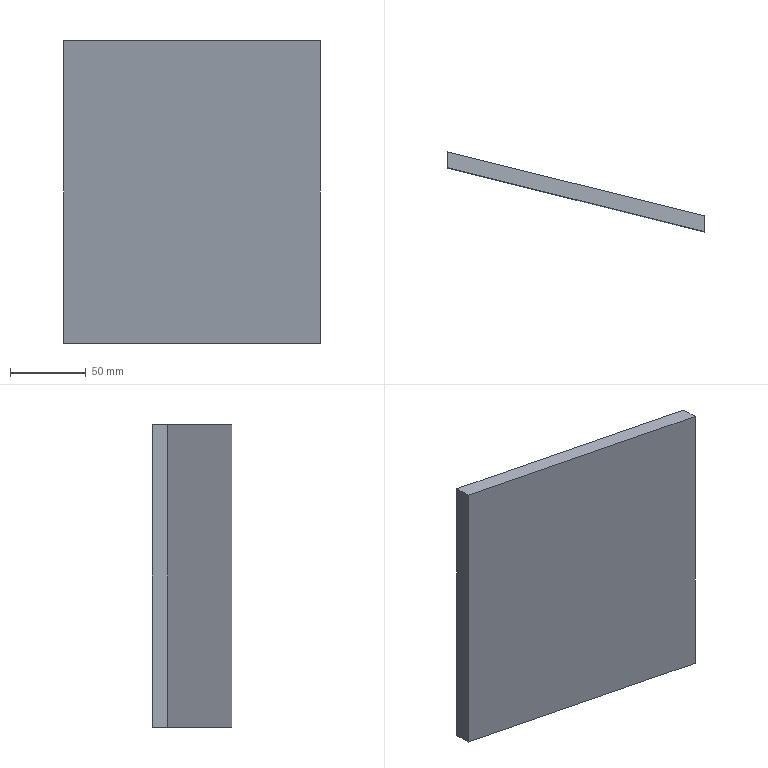Part | STEP file | 001-004-Feeding mechanism shaft slideway cover plate | 1 solid | 6 faces | box 170 x 52.886 x 200 mm | volume 357000 mm3 | plane 6
STEP:
#1=CARTESIAN_POINT('',(0.,0.,0.));
#2=DIRECTION('',(0.,0.,1.));
#3=DIRECTION('',(1.,0.,0.));
#4=AXIS2_PLACEMENT_3D('',#1,#2,#3);
#5=CARTESIAN_POINT('',(-170.,42.386,0.));
#6=VERTEX_POINT('',#5);
#7=CARTESIAN_POINT('',(0.,0.,0.));
#8=VERTEX_POINT('',#7);
#9=CARTESIAN_POINT('',(0.,0.,0.));
#10=DIRECTION('',(0.9703,-0.2419,0.));
#11=VECTOR('',#10,1.);
#12=LINE('',#9,#11);
#13=CARTESIAN_POINT('',(0.,0.,200.));
#14=DIRECTION('',(0.2419,0.9703,0.));
#15=DIRECTION('',(-0.9703,0.2419,0.));
#16=AXIS2_PLACEMENT_3D('',#13,#14,#15);
#17=PLANE('',#16);
#18=CARTESIAN_POINT('',(0.,-200.));
#19=DIRECTION('',(-1.,0.));
#20=VECTOR('',#19,1.);
#21=LINE('',#18,#20);
#22=(GEOMETRIC_REPRESENTATION_CONTEXT(2)PARAMETRIC_REPRESENTATION_CONTEXT()REPRESENTATION_CONTEXT('',''));
#23=DEFINITIONAL_REPRESENTATION('',(#21),#22);
#24=PCURVE('',#17,#23);
#25=CARTESIAN_POINT('',(0.,0.,0.));
#26=DIRECTION('',(0.,0.,-1.));
#27=DIRECTION('',(-1.,0.,0.));
#28=AXIS2_PLACEMENT_3D('',#25,#26,#27);
#29=PLANE('',#28);
#30=CARTESIAN_POINT('',(0.,0.));
#31=DIRECTION('',(-0.9703,-0.2419));
#32=VECTOR('',#31,1.);
#33=LINE('',#30,#32);
#34=(GEOMETRIC_REPRESENTATION_CONTEXT(2)PARAMETRIC_REPRESENTATION_CONTEXT()REPRESENTATION_CONTEXT('',''));
#35=DEFINITIONAL_REPRESENTATION('',(#33),#34);
#36=PCURVE('',#29,#35);
#37=SURFACE_CURVE('',#12,(#24,#36),.PCURVE_S1.);
#38=EDGE_CURVE('',#6,#8,#37,.T.);
#39=ORIENTED_EDGE('',*,*,#38,.T.);
#40=CARTESIAN_POINT('',(0.,0.,200.));
#41=VERTEX_POINT('',#40);
#42=CARTESIAN_POINT('',(0.,0.,200.));
#43=DIRECTION('',(0.,0.,-1.));
#44=VECTOR('',#43,1.);
#45=LINE('',#42,#44);
#46=CARTESIAN_POINT('',(0.,0.));
#47=DIRECTION('',(0.,-1.));
#48=VECTOR('',#47,1.);
#49=LINE('',#46,#48);
#50=(GEOMETRIC_REPRESENTATION_CONTEXT(2)PARAMETRIC_REPRESENTATION_CONTEXT()REPRESENTATION_CONTEXT('',''));
#51=DEFINITIONAL_REPRESENTATION('',(#49),#50);
#52=PCURVE('',#17,#51);
#53=CARTESIAN_POINT('',(0.,0.,200.));
#54=DIRECTION('',(-1.,0.,0.));
#55=DIRECTION('',(0.,0.,1.));
#56=AXIS2_PLACEMENT_3D('',#53,#54,#55);
#57=PLANE('',#56);
#58=CARTESIAN_POINT('',(0.,0.));
#59=DIRECTION('',(-1.,0.));
#60=VECTOR('',#59,1.);
#61=LINE('',#58,#60);
#62=(GEOMETRIC_REPRESENTATION_CONTEXT(2)PARAMETRIC_REPRESENTATION_CONTEXT()REPRESENTATION_CONTEXT('',''));
#63=DEFINITIONAL_REPRESENTATION('',(#61),#62);
#64=PCURVE('',#57,#63);
#65=SURFACE_CURVE('',#45,(#52,#64),.PCURVE_S1.);
#66=EDGE_CURVE('',#41,#8,#65,.T.);
#67=ORIENTED_EDGE('',*,*,#66,.F.);
#68=CARTESIAN_POINT('',(-170.,42.386,200.));
#69=VERTEX_POINT('',#68);
#70=CARTESIAN_POINT('',(0.,0.,200.));
#71=DIRECTION('',(0.9703,-0.2419,0.));
#72=VECTOR('',#71,1.);
#73=LINE('',#70,#72);
#74=CARTESIAN_POINT('',(0.,0.));
#75=DIRECTION('',(-1.,0.));
#76=VECTOR('',#75,1.);
#77=LINE('',#74,#76);
#78=(GEOMETRIC_REPRESENTATION_CONTEXT(2)PARAMETRIC_REPRESENTATION_CONTEXT()REPRESENTATION_CONTEXT('',''));
#79=DEFINITIONAL_REPRESENTATION('',(#77),#78);
#80=PCURVE('',#17,#79);
#81=CARTESIAN_POINT('',(0.,0.,200.));
#82=DIRECTION('',(0.,0.,-1.));
#83=DIRECTION('',(-1.,0.,0.));
#84=AXIS2_PLACEMENT_3D('',#81,#82,#83);
#85=PLANE('',#84);
#86=CARTESIAN_POINT('',(0.,0.));
#87=DIRECTION('',(-0.9703,-0.2419));
#88=VECTOR('',#87,1.);
#89=LINE('',#86,#88);
#90=(GEOMETRIC_REPRESENTATION_CONTEXT(2)PARAMETRIC_REPRESENTATION_CONTEXT()REPRESENTATION_CONTEXT('',''));
#91=DEFINITIONAL_REPRESENTATION('',(#89),#90);
#92=PCURVE('',#85,#91);
#93=SURFACE_CURVE('',#73,(#80,#92),.PCURVE_S1.);
#94=EDGE_CURVE('',#69,#41,#93,.T.);
#95=ORIENTED_EDGE('',*,*,#94,.F.);
#96=CARTESIAN_POINT('',(-170.,42.386,200.));
#97=DIRECTION('',(0.,0.,-1.));
#98=VECTOR('',#97,1.);
#99=LINE('',#96,#98);
#100=CARTESIAN_POINT('',(175.204,0.));
#101=DIRECTION('',(0.,-1.));
#102=VECTOR('',#101,1.);
#103=LINE('',#100,#102);
#104=(GEOMETRIC_REPRESENTATION_CONTEXT(2)PARAMETRIC_REPRESENTATION_CONTEXT()REPRESENTATION_CONTEXT('',''));
#105=DEFINITIONAL_REPRESENTATION('',(#103),#104);
#106=PCURVE('',#17,#105);
#107=CARTESIAN_POINT('',(-170.,42.386,200.));
#108=DIRECTION('',(1.,0.,0.));
#109=DIRECTION('',(0.,0.,-1.));
#110=AXIS2_PLACEMENT_3D('',#107,#108,#109);
#111=PLANE('',#110);
#112=CARTESIAN_POINT('',(0.,0.));
#113=DIRECTION('',(1.,0.));
#114=VECTOR('',#113,1.);
#115=LINE('',#112,#114);
#116=(GEOMETRIC_REPRESENTATION_CONTEXT(2)PARAMETRIC_REPRESENTATION_CONTEXT()REPRESENTATION_CONTEXT('',''));
#117=DEFINITIONAL_REPRESENTATION('',(#115),#116);
#118=PCURVE('',#111,#117);
#119=SURFACE_CURVE('',#99,(#106,#118),.PCURVE_S1.);
#120=EDGE_CURVE('',#69,#6,#119,.T.);
#121=ORIENTED_EDGE('',*,*,#120,.T.);
#122=EDGE_LOOP('',(#39,#67,#95,#121));
#123=FACE_BOUND('',#122,.T.);
#124=ADVANCED_FACE('',(#123),#17,.F.);
#125=CARTESIAN_POINT('',(0.,10.5,0.));
#126=VERTEX_POINT('',#125);
#127=CARTESIAN_POINT('',(0.,0.,0.));
#128=DIRECTION('',(0.,1.,0.));
#129=VECTOR('',#128,1.);
#130=LINE('',#127,#129);
#131=CARTESIAN_POINT('',(-200.,0.));
#132=DIRECTION('',(0.,1.));
#133=VECTOR('',#132,1.);
#134=LINE('',#131,#133);
#135=(GEOMETRIC_REPRESENTATION_CONTEXT(2)PARAMETRIC_REPRESENTATION_CONTEXT()REPRESENTATION_CONTEXT('',''));
#136=DEFINITIONAL_REPRESENTATION('',(#134),#135);
#137=PCURVE('',#57,#136);
#138=CARTESIAN_POINT('',(0.,0.));
#139=DIRECTION('',(0.,1.));
#140=VECTOR('',#139,1.);
#141=LINE('',#138,#140);
#142=(GEOMETRIC_REPRESENTATION_CONTEXT(2)PARAMETRIC_REPRESENTATION_CONTEXT()REPRESENTATION_CONTEXT('',''));
#143=DEFINITIONAL_REPRESENTATION('',(#141),#142);
#144=PCURVE('',#29,#143);
#145=SURFACE_CURVE('',#130,(#137,#144),.PCURVE_S1.);
#146=EDGE_CURVE('',#8,#126,#145,.T.);
#147=ORIENTED_EDGE('',*,*,#146,.T.);
#148=CARTESIAN_POINT('',(0.,10.5,200.));
#149=VERTEX_POINT('',#148);
#150=CARTESIAN_POINT('',(0.,10.5,200.));
#151=DIRECTION('',(0.,0.,-1.));
#152=VECTOR('',#151,1.);
#153=LINE('',#150,#152);
#154=CARTESIAN_POINT('',(0.,10.5));
#155=DIRECTION('',(-1.,0.));
#156=VECTOR('',#155,1.);
#157=LINE('',#154,#156);
#158=(GEOMETRIC_REPRESENTATION_CONTEXT(2)PARAMETRIC_REPRESENTATION_CONTEXT()REPRESENTATION_CONTEXT('',''));
#159=DEFINITIONAL_REPRESENTATION('',(#157),#158);
#160=PCURVE('',#57,#159);
#161=CARTESIAN_POINT('',(0.,10.5,200.));
#162=DIRECTION('',(-0.2419,-0.9703,0.));
#163=DIRECTION('',(0.9703,-0.2419,0.));
#164=AXIS2_PLACEMENT_3D('',#161,#162,#163);
#165=PLANE('',#164);
#166=CARTESIAN_POINT('',(0.,0.));
#167=DIRECTION('',(0.,-1.));
#168=VECTOR('',#167,1.);
#169=LINE('',#166,#168);
#170=(GEOMETRIC_REPRESENTATION_CONTEXT(2)PARAMETRIC_REPRESENTATION_CONTEXT()REPRESENTATION_CONTEXT('',''));
#171=DEFINITIONAL_REPRESENTATION('',(#169),#170);
#172=PCURVE('',#165,#171);
#173=SURFACE_CURVE('',#153,(#160,#172),.PCURVE_S1.);
#174=EDGE_CURVE('',#149,#126,#173,.T.);
#175=ORIENTED_EDGE('',*,*,#174,.F.);
#176=CARTESIAN_POINT('',(0.,0.,200.));
#177=DIRECTION('',(0.,1.,0.));
#178=VECTOR('',#177,1.);
#179=LINE('',#176,#178);
#180=CARTESIAN_POINT('',(0.,0.));
#181=DIRECTION('',(0.,1.));
#182=VECTOR('',#181,1.);
#183=LINE('',#180,#182);
#184=(GEOMETRIC_REPRESENTATION_CONTEXT(2)PARAMETRIC_REPRESENTATION_CONTEXT()REPRESENTATION_CONTEXT('',''));
#185=DEFINITIONAL_REPRESENTATION('',(#183),#184);
#186=PCURVE('',#57,#185);
#187=CARTESIAN_POINT('',(0.,0.));
#188=DIRECTION('',(0.,1.));
#189=VECTOR('',#188,1.);
#190=LINE('',#187,#189);
#191=(GEOMETRIC_REPRESENTATION_CONTEXT(2)PARAMETRIC_REPRESENTATION_CONTEXT()REPRESENTATION_CONTEXT('',''));
#192=DEFINITIONAL_REPRESENTATION('',(#190),#191);
#193=PCURVE('',#85,#192);
#194=SURFACE_CURVE('',#179,(#186,#193),.PCURVE_S1.);
#195=EDGE_CURVE('',#41,#149,#194,.T.);
#196=ORIENTED_EDGE('',*,*,#195,.F.);
#197=ORIENTED_EDGE('',*,*,#66,.T.);
#198=EDGE_LOOP('',(#147,#175,#196,#197));
#199=FACE_BOUND('',#198,.T.);
#200=ADVANCED_FACE('',(#199),#57,.F.);
#201=CARTESIAN_POINT('',(-170.,52.886,0.));
#202=VERTEX_POINT('',#201);
#203=CARTESIAN_POINT('',(0.,10.5,0.));
#204=DIRECTION('',(-0.9703,0.2419,0.));
#205=VECTOR('',#204,1.);
#206=LINE('',#203,#205);
#207=CARTESIAN_POINT('',(0.,-200.));
#208=DIRECTION('',(-1.,0.));
#209=VECTOR('',#208,1.);
#210=LINE('',#207,#209);
#211=(GEOMETRIC_REPRESENTATION_CONTEXT(2)PARAMETRIC_REPRESENTATION_CONTEXT()REPRESENTATION_CONTEXT('',''));
#212=DEFINITIONAL_REPRESENTATION('',(#210),#211);
#213=PCURVE('',#165,#212);
#214=CARTESIAN_POINT('',(0.,10.5));
#215=DIRECTION('',(0.9703,0.2419));
#216=VECTOR('',#215,1.);
#217=LINE('',#214,#216);
#218=(GEOMETRIC_REPRESENTATION_CONTEXT(2)PARAMETRIC_REPRESENTATION_CONTEXT()REPRESENTATION_CONTEXT('',''));
#219=DEFINITIONAL_REPRESENTATION('',(#217),#218);
#220=PCURVE('',#29,#219);
#221=SURFACE_CURVE('',#206,(#213,#220),.PCURVE_S1.);
#222=EDGE_CURVE('',#126,#202,#221,.T.);
#223=ORIENTED_EDGE('',*,*,#222,.T.);
#224=CARTESIAN_POINT('',(-170.,52.886,200.));
#225=VERTEX_POINT('',#224);
#226=CARTESIAN_POINT('',(-170.,52.886,200.));
#227=DIRECTION('',(0.,0.,-1.));
#228=VECTOR('',#227,1.);
#229=LINE('',#226,#228);
#230=CARTESIAN_POINT('',(-175.204,0.));
#231=DIRECTION('',(0.,-1.));
#232=VECTOR('',#231,1.);
#233=LINE('',#230,#232);
#234=(GEOMETRIC_REPRESENTATION_CONTEXT(2)PARAMETRIC_REPRESENTATION_CONTEXT()REPRESENTATION_CONTEXT('',''));
#235=DEFINITIONAL_REPRESENTATION('',(#233),#234);
#236=PCURVE('',#165,#235);
#237=CARTESIAN_POINT('',(0.,10.5));
#238=DIRECTION('',(1.,0.));
#239=VECTOR('',#238,1.);
#240=LINE('',#237,#239);
#241=(GEOMETRIC_REPRESENTATION_CONTEXT(2)PARAMETRIC_REPRESENTATION_CONTEXT()REPRESENTATION_CONTEXT('',''));
#242=DEFINITIONAL_REPRESENTATION('',(#240),#241);
#243=PCURVE('',#111,#242);
#244=SURFACE_CURVE('',#229,(#236,#243),.PCURVE_S1.);
#245=EDGE_CURVE('',#225,#202,#244,.T.);
#246=ORIENTED_EDGE('',*,*,#245,.F.);
#247=CARTESIAN_POINT('',(0.,10.5,200.));
#248=DIRECTION('',(-0.9703,0.2419,0.));
#249=VECTOR('',#248,1.);
#250=LINE('',#247,#249);
#251=CARTESIAN_POINT('',(0.,0.));
#252=DIRECTION('',(-1.,0.));
#253=VECTOR('',#252,1.);
#254=LINE('',#251,#253);
#255=(GEOMETRIC_REPRESENTATION_CONTEXT(2)PARAMETRIC_REPRESENTATION_CONTEXT()REPRESENTATION_CONTEXT('',''));
#256=DEFINITIONAL_REPRESENTATION('',(#254),#255);
#257=PCURVE('',#165,#256);
#258=CARTESIAN_POINT('',(0.,10.5));
#259=DIRECTION('',(0.9703,0.2419));
#260=VECTOR('',#259,1.);
#261=LINE('',#258,#260);
#262=(GEOMETRIC_REPRESENTATION_CONTEXT(2)PARAMETRIC_REPRESENTATION_CONTEXT()REPRESENTATION_CONTEXT('',''));
#263=DEFINITIONAL_REPRESENTATION('',(#261),#262);
#264=PCURVE('',#85,#263);
#265=SURFACE_CURVE('',#250,(#257,#264),.PCURVE_S1.);
#266=EDGE_CURVE('',#149,#225,#265,.T.);
#267=ORIENTED_EDGE('',*,*,#266,.F.);
#268=ORIENTED_EDGE('',*,*,#174,.T.);
#269=EDGE_LOOP('',(#223,#246,#267,#268));
#270=FACE_BOUND('',#269,.T.);
#271=ADVANCED_FACE('',(#270),#165,.F.);
#272=CARTESIAN_POINT('',(-170.,42.386,0.));
#273=DIRECTION('',(0.,-1.,0.));
#274=VECTOR('',#273,1.);
#275=LINE('',#272,#274);
#276=CARTESIAN_POINT('',(200.,0.));
#277=DIRECTION('',(0.,-1.));
#278=VECTOR('',#277,1.);
#279=LINE('',#276,#278);
#280=(GEOMETRIC_REPRESENTATION_CONTEXT(2)PARAMETRIC_REPRESENTATION_CONTEXT()REPRESENTATION_CONTEXT('',''));
#281=DEFINITIONAL_REPRESENTATION('',(#279),#280);
#282=PCURVE('',#111,#281);
#283=CARTESIAN_POINT('',(170.,42.386));
#284=DIRECTION('',(0.,-1.));
#285=VECTOR('',#284,1.);
#286=LINE('',#283,#285);
#287=(GEOMETRIC_REPRESENTATION_CONTEXT(2)PARAMETRIC_REPRESENTATION_CONTEXT()REPRESENTATION_CONTEXT('',''));
#288=DEFINITIONAL_REPRESENTATION('',(#286),#287);
#289=PCURVE('',#29,#288);
#290=SURFACE_CURVE('',#275,(#282,#289),.PCURVE_S1.);
#291=EDGE_CURVE('',#202,#6,#290,.T.);
#292=ORIENTED_EDGE('',*,*,#291,.T.);
#293=ORIENTED_EDGE('',*,*,#120,.F.);
#294=CARTESIAN_POINT('',(-170.,42.386,200.));
#295=DIRECTION('',(0.,-1.,0.));
#296=VECTOR('',#295,1.);
#297=LINE('',#294,#296);
#298=CARTESIAN_POINT('',(0.,0.));
#299=DIRECTION('',(0.,-1.));
#300=VECTOR('',#299,1.);
#301=LINE('',#298,#300);
#302=(GEOMETRIC_REPRESENTATION_CONTEXT(2)PARAMETRIC_REPRESENTATION_CONTEXT()REPRESENTATION_CONTEXT('',''));
#303=DEFINITIONAL_REPRESENTATION('',(#301),#302);
#304=PCURVE('',#111,#303);
#305=CARTESIAN_POINT('',(170.,42.386));
#306=DIRECTION('',(0.,-1.));
#307=VECTOR('',#306,1.);
#308=LINE('',#305,#307);
#309=(GEOMETRIC_REPRESENTATION_CONTEXT(2)PARAMETRIC_REPRESENTATION_CONTEXT()REPRESENTATION_CONTEXT('',''));
#310=DEFINITIONAL_REPRESENTATION('',(#308),#309);
#311=PCURVE('',#85,#310);
#312=SURFACE_CURVE('',#297,(#304,#311),.PCURVE_S1.);
#313=EDGE_CURVE('',#225,#69,#312,.T.);
#314=ORIENTED_EDGE('',*,*,#313,.F.);
#315=ORIENTED_EDGE('',*,*,#245,.T.);
#316=EDGE_LOOP('',(#292,#293,#314,#315));
#317=FACE_BOUND('',#316,.T.);
#318=ADVANCED_FACE('',(#317),#111,.F.);
#319=ORIENTED_EDGE('',*,*,#94,.T.);
#320=ORIENTED_EDGE('',*,*,#195,.T.);
#321=ORIENTED_EDGE('',*,*,#266,.T.);
#322=ORIENTED_EDGE('',*,*,#313,.T.);
#323=EDGE_LOOP('',(#319,#320,#321,#322));
#324=FACE_BOUND('',#323,.T.);
#325=ADVANCED_FACE('',(#324),#85,.F.);
#326=ORIENTED_EDGE('',*,*,#38,.F.);
#327=ORIENTED_EDGE('',*,*,#291,.F.);
#328=ORIENTED_EDGE('',*,*,#222,.F.);
#329=ORIENTED_EDGE('',*,*,#146,.F.);
#330=EDGE_LOOP('',(#326,#327,#328,#329));
#331=FACE_BOUND('',#330,.T.);
#332=ADVANCED_FACE('',(#331),#29,.T.);
#333=CLOSED_SHELL('',(#124,#200,#271,#318,#325,#332));
#334=MANIFOLD_SOLID_BREP('',#333);
#335=(LENGTH_UNIT()NAMED_UNIT(*)SI_UNIT(.MILLI.,.METRE.));
#336=UNCERTAINTY_MEASURE_WITH_UNIT(LENGTH_MEASURE(0.0000001),#335,'','');
#337=(NAMED_UNIT(*)PLANE_ANGLE_UNIT()SI_UNIT($,.RADIAN.));
#338=(NAMED_UNIT(*)SI_UNIT($,.STERADIAN.)SOLID_ANGLE_UNIT());
#339=(GEOMETRIC_REPRESENTATION_CONTEXT(3)GLOBAL_UNCERTAINTY_ASSIGNED_CONTEXT((#336))GLOBAL_UNIT_ASSIGNED_CONTEXT((#335,#337,#338))REPRESENTATION_CONTEXT('',''));
#340=ADVANCED_BREP_SHAPE_REPRESENTATION('',(#4,#334),#339);